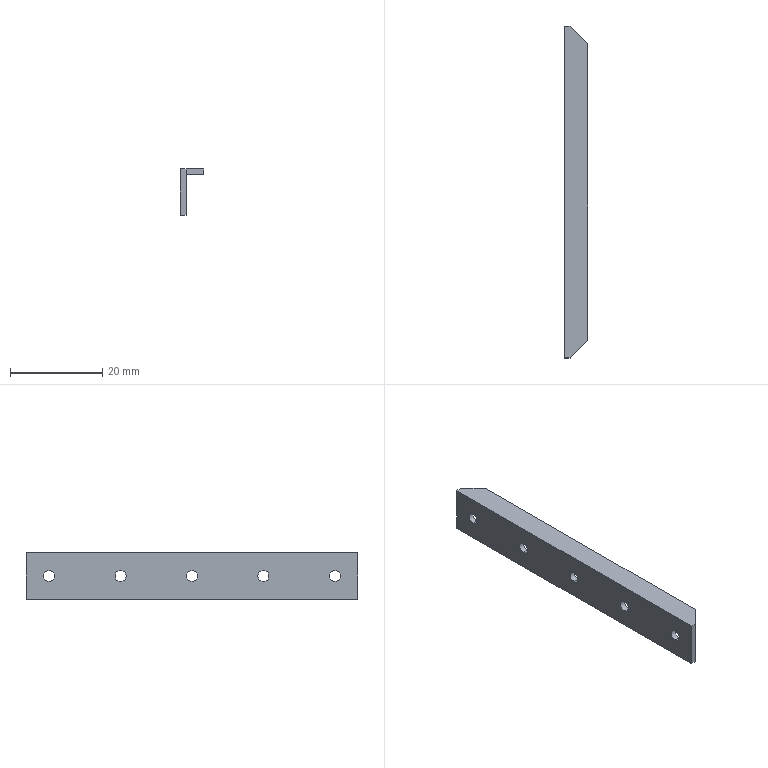Part | SolidWorks | features BaseBody 1 | 1 solid | 20 faces | box 5 x 72 x 10 mm | volume 1148 mm3 | cylinder 10 | plane 10 | commonest cylinder face diameters 2.4 x10
STEP:
#1=CARTESIAN_POINT('',(0.,20.5,-6.2));
#2=VERTEX_POINT('',#1);
#3=CARTESIAN_POINT('',(0.,20.5,-3.8));
#4=VERTEX_POINT('',#3);
#5=CARTESIAN_POINT('',(0.,20.5,-5.));
#6=DIRECTION('',(-1.,0.,0.));
#7=DIRECTION('',(0.,0.,-1.));
#8=AXIS2_PLACEMENT_3D('',#5,#6,#7);
#9=CIRCLE('',#8,1.2);
#10=EDGE_CURVE('',#2,#4,#9,.T.);
#11=ORIENTED_EDGE('',*,*,#10,.T.);
#12=CARTESIAN_POINT('',(1.2,20.5,-3.8));
#13=VERTEX_POINT('',#12);
#14=CARTESIAN_POINT('',(0.,20.5,-3.8));
#15=DIRECTION('',(1.,0.,0.));
#16=VECTOR('',#15,1000.);
#17=LINE('',#14,#16);
#18=EDGE_CURVE('',#4,#13,#17,.T.);
#19=ORIENTED_EDGE('',*,*,#18,.T.);
#20=CARTESIAN_POINT('',(1.2,20.5,-6.2));
#21=VERTEX_POINT('',#20);
#22=CARTESIAN_POINT('',(1.2,20.5,-5.));
#23=DIRECTION('',(1.,0.,0.));
#24=DIRECTION('',(0.,0.,-1.));
#25=AXIS2_PLACEMENT_3D('',#22,#23,#24);
#26=CIRCLE('',#25,1.2);
#27=EDGE_CURVE('',#13,#21,#26,.T.);
#28=ORIENTED_EDGE('',*,*,#27,.T.);
#29=CARTESIAN_POINT('',(0.,20.5,-6.2));
#30=DIRECTION('',(1.,0.,0.));
#31=VECTOR('',#30,1000.);
#32=LINE('',#29,#31);
#33=EDGE_CURVE('',#2,#21,#32,.T.);
#34=ORIENTED_EDGE('',*,*,#33,.F.);
#35=EDGE_LOOP('',(#11,#19,#28,#34));
#36=FACE_OUTER_BOUND('',#35,.T.);
#37=CARTESIAN_POINT('',(0.,20.5,-5.));
#38=DIRECTION('',(1.,0.,0.));
#39=DIRECTION('',(0.,0.,-1.));
#40=AXIS2_PLACEMENT_3D('',#37,#38,#39);
#41=CYLINDRICAL_SURFACE('',#40,1.2);
#42=ADVANCED_FACE('',(#36),#41,.F.);
#43=CARTESIAN_POINT('',(0.,67.,-6.2));
#44=VERTEX_POINT('',#43);
#45=CARTESIAN_POINT('',(0.,67.,-3.8));
#46=VERTEX_POINT('',#45);
#47=CARTESIAN_POINT('',(0.,67.,-5.));
#48=DIRECTION('',(-1.,0.,0.));
#49=DIRECTION('',(0.,0.,-1.));
#50=AXIS2_PLACEMENT_3D('',#47,#48,#49);
#51=CIRCLE('',#50,1.2);
#52=EDGE_CURVE('',#44,#46,#51,.T.);
#53=ORIENTED_EDGE('',*,*,#52,.T.);
#54=CARTESIAN_POINT('',(1.2,67.,-3.8));
#55=VERTEX_POINT('',#54);
#56=CARTESIAN_POINT('',(0.,67.,-3.8));
#57=DIRECTION('',(1.,0.,0.));
#58=VECTOR('',#57,1000.);
#59=LINE('',#56,#58);
#60=EDGE_CURVE('',#46,#55,#59,.T.);
#61=ORIENTED_EDGE('',*,*,#60,.T.);
#62=CARTESIAN_POINT('',(1.2,67.,-6.2));
#63=VERTEX_POINT('',#62);
#64=CARTESIAN_POINT('',(1.2,67.,-5.));
#65=DIRECTION('',(1.,0.,0.));
#66=DIRECTION('',(0.,0.,-1.));
#67=AXIS2_PLACEMENT_3D('',#64,#65,#66);
#68=CIRCLE('',#67,1.2);
#69=EDGE_CURVE('',#55,#63,#68,.T.);
#70=ORIENTED_EDGE('',*,*,#69,.T.);
#71=CARTESIAN_POINT('',(0.,67.,-6.2));
#72=DIRECTION('',(1.,0.,0.));
#73=VECTOR('',#72,1000.);
#74=LINE('',#71,#73);
#75=EDGE_CURVE('',#44,#63,#74,.T.);
#76=ORIENTED_EDGE('',*,*,#75,.F.);
#77=EDGE_LOOP('',(#53,#61,#70,#76));
#78=FACE_OUTER_BOUND('',#77,.T.);
#79=CARTESIAN_POINT('',(0.,67.,-5.));
#80=DIRECTION('',(1.,0.,0.));
#81=DIRECTION('',(0.,0.,-1.));
#82=AXIS2_PLACEMENT_3D('',#79,#80,#81);
#83=CYLINDRICAL_SURFACE('',#82,1.2);
#84=ADVANCED_FACE('',(#78),#83,.F.);
#85=CARTESIAN_POINT('',(0.,5.,-6.2));
#86=VERTEX_POINT('',#85);
#87=CARTESIAN_POINT('',(0.,5.,-3.8));
#88=VERTEX_POINT('',#87);
#89=CARTESIAN_POINT('',(0.,5.,-5.));
#90=DIRECTION('',(-1.,0.,0.));
#91=DIRECTION('',(0.,0.,-1.));
#92=AXIS2_PLACEMENT_3D('',#89,#90,#91);
#93=CIRCLE('',#92,1.2);
#94=EDGE_CURVE('',#86,#88,#93,.T.);
#95=ORIENTED_EDGE('',*,*,#94,.T.);
#96=CARTESIAN_POINT('',(1.2,5.,-3.8));
#97=VERTEX_POINT('',#96);
#98=CARTESIAN_POINT('',(0.,5.,-3.8));
#99=DIRECTION('',(1.,0.,0.));
#100=VECTOR('',#99,1000.);
#101=LINE('',#98,#100);
#102=EDGE_CURVE('',#88,#97,#101,.T.);
#103=ORIENTED_EDGE('',*,*,#102,.T.);
#104=CARTESIAN_POINT('',(1.2,5.,-6.2));
#105=VERTEX_POINT('',#104);
#106=CARTESIAN_POINT('',(1.2,5.,-5.));
#107=DIRECTION('',(1.,0.,0.));
#108=DIRECTION('',(0.,0.,-1.));
#109=AXIS2_PLACEMENT_3D('',#106,#107,#108);
#110=CIRCLE('',#109,1.2);
#111=EDGE_CURVE('',#97,#105,#110,.T.);
#112=ORIENTED_EDGE('',*,*,#111,.T.);
#113=CARTESIAN_POINT('',(0.,5.,-6.2));
#114=DIRECTION('',(1.,0.,0.));
#115=VECTOR('',#114,1000.);
#116=LINE('',#113,#115);
#117=EDGE_CURVE('',#86,#105,#116,.T.);
#118=ORIENTED_EDGE('',*,*,#117,.F.);
#119=EDGE_LOOP('',(#95,#103,#112,#118));
#120=FACE_OUTER_BOUND('',#119,.T.);
#121=CARTESIAN_POINT('',(0.,5.,-5.));
#122=DIRECTION('',(1.,0.,0.));
#123=DIRECTION('',(0.,0.,-1.));
#124=AXIS2_PLACEMENT_3D('',#121,#122,#123);
#125=CYLINDRICAL_SURFACE('',#124,1.2);
#126=ADVANCED_FACE('',(#120),#125,.F.);
#127=CARTESIAN_POINT('',(0.,36.,-6.2));
#128=VERTEX_POINT('',#127);
#129=CARTESIAN_POINT('',(0.,36.,-3.8));
#130=VERTEX_POINT('',#129);
#131=CARTESIAN_POINT('',(0.,36.,-5.));
#132=DIRECTION('',(-1.,0.,0.));
#133=DIRECTION('',(0.,0.,-1.));
#134=AXIS2_PLACEMENT_3D('',#131,#132,#133);
#135=CIRCLE('',#134,1.2);
#136=EDGE_CURVE('',#128,#130,#135,.T.);
#137=ORIENTED_EDGE('',*,*,#136,.T.);
#138=CARTESIAN_POINT('',(1.2,36.,-3.8));
#139=VERTEX_POINT('',#138);
#140=CARTESIAN_POINT('',(0.,36.,-3.8));
#141=DIRECTION('',(1.,0.,0.));
#142=VECTOR('',#141,1000.);
#143=LINE('',#140,#142);
#144=EDGE_CURVE('',#130,#139,#143,.T.);
#145=ORIENTED_EDGE('',*,*,#144,.T.);
#146=CARTESIAN_POINT('',(1.2,36.,-6.2));
#147=VERTEX_POINT('',#146);
#148=CARTESIAN_POINT('',(1.2,36.,-5.));
#149=DIRECTION('',(1.,0.,0.));
#150=DIRECTION('',(0.,0.,-1.));
#151=AXIS2_PLACEMENT_3D('',#148,#149,#150);
#152=CIRCLE('',#151,1.2);
#153=EDGE_CURVE('',#139,#147,#152,.T.);
#154=ORIENTED_EDGE('',*,*,#153,.T.);
#155=CARTESIAN_POINT('',(0.,36.,-6.2));
#156=DIRECTION('',(1.,0.,0.));
#157=VECTOR('',#156,1000.);
#158=LINE('',#155,#157);
#159=EDGE_CURVE('',#128,#147,#158,.T.);
#160=ORIENTED_EDGE('',*,*,#159,.F.);
#161=EDGE_LOOP('',(#137,#145,#154,#160));
#162=FACE_OUTER_BOUND('',#161,.T.);
#163=CARTESIAN_POINT('',(0.,36.,-5.));
#164=DIRECTION('',(1.,0.,0.));
#165=DIRECTION('',(0.,0.,-1.));
#166=AXIS2_PLACEMENT_3D('',#163,#164,#165);
#167=CYLINDRICAL_SURFACE('',#166,1.2);
#168=ADVANCED_FACE('',(#162),#167,.F.);
#169=CARTESIAN_POINT('',(0.,51.5,-6.2));
#170=VERTEX_POINT('',#169);
#171=CARTESIAN_POINT('',(0.,51.5,-3.8));
#172=VERTEX_POINT('',#171);
#173=CARTESIAN_POINT('',(0.,51.5,-5.));
#174=DIRECTION('',(-1.,0.,0.));
#175=DIRECTION('',(0.,0.,-1.));
#176=AXIS2_PLACEMENT_3D('',#173,#174,#175);
#177=CIRCLE('',#176,1.2);
#178=EDGE_CURVE('',#170,#172,#177,.T.);
#179=ORIENTED_EDGE('',*,*,#178,.T.);
#180=CARTESIAN_POINT('',(1.2,51.5,-3.8));
#181=VERTEX_POINT('',#180);
#182=CARTESIAN_POINT('',(0.,51.5,-3.8));
#183=DIRECTION('',(1.,0.,0.));
#184=VECTOR('',#183,1000.);
#185=LINE('',#182,#184);
#186=EDGE_CURVE('',#172,#181,#185,.T.);
#187=ORIENTED_EDGE('',*,*,#186,.T.);
#188=CARTESIAN_POINT('',(1.2,51.5,-6.2));
#189=VERTEX_POINT('',#188);
#190=CARTESIAN_POINT('',(1.2,51.5,-5.));
#191=DIRECTION('',(1.,0.,0.));
#192=DIRECTION('',(0.,0.,-1.));
#193=AXIS2_PLACEMENT_3D('',#190,#191,#192);
#194=CIRCLE('',#193,1.2);
#195=EDGE_CURVE('',#181,#189,#194,.T.);
#196=ORIENTED_EDGE('',*,*,#195,.T.);
#197=CARTESIAN_POINT('',(0.,51.5,-6.2));
#198=DIRECTION('',(1.,0.,0.));
#199=VECTOR('',#198,1000.);
#200=LINE('',#197,#199);
#201=EDGE_CURVE('',#170,#189,#200,.T.);
#202=ORIENTED_EDGE('',*,*,#201,.F.);
#203=EDGE_LOOP('',(#179,#187,#196,#202));
#204=FACE_OUTER_BOUND('',#203,.T.);
#205=CARTESIAN_POINT('',(0.,51.5,-5.));
#206=DIRECTION('',(1.,0.,0.));
#207=DIRECTION('',(0.,0.,-1.));
#208=AXIS2_PLACEMENT_3D('',#205,#206,#207);
#209=CYLINDRICAL_SURFACE('',#208,1.2);
#210=ADVANCED_FACE('',(#204),#209,.F.);
#211=ORIENTED_EDGE('',*,*,#18,.F.);
#212=CARTESIAN_POINT('',(0.,20.5,-5.));
#213=DIRECTION('',(-1.,0.,0.));
#214=DIRECTION('',(0.,0.,-1.));
#215=AXIS2_PLACEMENT_3D('',#212,#213,#214);
#216=CIRCLE('',#215,1.2);
#217=EDGE_CURVE('',#4,#2,#216,.T.);
#218=ORIENTED_EDGE('',*,*,#217,.T.);
#219=ORIENTED_EDGE('',*,*,#33,.T.);
#220=CARTESIAN_POINT('',(1.2,20.5,-5.));
#221=DIRECTION('',(1.,0.,0.));
#222=DIRECTION('',(0.,0.,-1.));
#223=AXIS2_PLACEMENT_3D('',#220,#221,#222);
#224=CIRCLE('',#223,1.2);
#225=EDGE_CURVE('',#21,#13,#224,.T.);
#226=ORIENTED_EDGE('',*,*,#225,.T.);
#227=EDGE_LOOP('',(#211,#218,#219,#226));
#228=FACE_OUTER_BOUND('',#227,.T.);
#229=CARTESIAN_POINT('',(0.,20.5,-5.));
#230=DIRECTION('',(1.,0.,0.));
#231=DIRECTION('',(0.,0.,-1.));
#232=AXIS2_PLACEMENT_3D('',#229,#230,#231);
#233=CYLINDRICAL_SURFACE('',#232,1.2);
#234=ADVANCED_FACE('',(#228),#233,.F.);
#235=CARTESIAN_POINT('',(1.2,67.,-5.));
#236=DIRECTION('',(1.,0.,0.));
#237=DIRECTION('',(0.,0.,-1.));
#238=AXIS2_PLACEMENT_3D('',#235,#236,#237);
#239=CIRCLE('',#238,1.2);
#240=EDGE_CURVE('',#63,#55,#239,.T.);
#241=ORIENTED_EDGE('',*,*,#240,.F.);
#242=ORIENTED_EDGE('',*,*,#69,.F.);
#243=EDGE_LOOP('',(#241,#242));
#244=FACE_BOUND('',#243,.T.);
#245=CARTESIAN_POINT('',(1.2,5.,-5.));
#246=DIRECTION('',(1.,0.,0.));
#247=DIRECTION('',(0.,0.,-1.));
#248=AXIS2_PLACEMENT_3D('',#245,#246,#247);
#249=CIRCLE('',#248,1.2);
#250=EDGE_CURVE('',#105,#97,#249,.T.);
#251=ORIENTED_EDGE('',*,*,#250,.F.);
#252=ORIENTED_EDGE('',*,*,#111,.F.);
#253=EDGE_LOOP('',(#251,#252));
#254=FACE_BOUND('',#253,.T.);
#255=CARTESIAN_POINT('',(1.2,36.,-5.));
#256=DIRECTION('',(1.,0.,0.));
#257=DIRECTION('',(0.,0.,-1.));
#258=AXIS2_PLACEMENT_3D('',#255,#256,#257);
#259=CIRCLE('',#258,1.2);
#260=EDGE_CURVE('',#147,#139,#259,.T.);
#261=ORIENTED_EDGE('',*,*,#260,.F.);
#262=ORIENTED_EDGE('',*,*,#153,.F.);
#263=EDGE_LOOP('',(#261,#262));
#264=FACE_BOUND('',#263,.T.);
#265=CARTESIAN_POINT('',(1.2,51.5,-5.));
#266=DIRECTION('',(1.,0.,0.));
#267=DIRECTION('',(0.,0.,-1.));
#268=AXIS2_PLACEMENT_3D('',#265,#266,#267);
#269=CIRCLE('',#268,1.2);
#270=EDGE_CURVE('',#189,#181,#269,.T.);
#271=ORIENTED_EDGE('',*,*,#270,.F.);
#272=ORIENTED_EDGE('',*,*,#195,.F.);
#273=EDGE_LOOP('',(#271,#272));
#274=FACE_BOUND('',#273,.T.);
#275=ORIENTED_EDGE('',*,*,#225,.F.);
#276=ORIENTED_EDGE('',*,*,#27,.F.);
#277=EDGE_LOOP('',(#275,#276));
#278=FACE_BOUND('',#277,.T.);
#279=CARTESIAN_POINT('',(1.2,72.,-10.));
#280=VERTEX_POINT('',#279);
#281=CARTESIAN_POINT('',(1.2,0.,-10.));
#282=VERTEX_POINT('',#281);
#283=CARTESIAN_POINT('',(1.2,36.,-10.));
#284=DIRECTION('',(0.,-1.,0.));
#285=VECTOR('',#284,1000.);
#286=LINE('',#283,#285);
#287=EDGE_CURVE('',#280,#282,#286,.T.);
#288=ORIENTED_EDGE('',*,*,#287,.F.);
#289=CARTESIAN_POINT('',(1.2,72.,-1.2));
#290=VERTEX_POINT('',#289);
#291=CARTESIAN_POINT('',(1.2,72.,-5.6));
#292=DIRECTION('',(0.,0.,-1.));
#293=VECTOR('',#292,1000.);
#294=LINE('',#291,#293);
#295=EDGE_CURVE('',#290,#280,#294,.T.);
#296=ORIENTED_EDGE('',*,*,#295,.F.);
#297=CARTESIAN_POINT('',(1.2,0.,-1.2));
#298=VERTEX_POINT('',#297);
#299=CARTESIAN_POINT('',(1.2,36.,-1.2));
#300=DIRECTION('',(0.,1.,0.));
#301=VECTOR('',#300,1000.);
#302=LINE('',#299,#301);
#303=EDGE_CURVE('',#298,#290,#302,.T.);
#304=ORIENTED_EDGE('',*,*,#303,.F.);
#305=CARTESIAN_POINT('',(1.2,0.,-5.6));
#306=DIRECTION('',(0.,0.,1.));
#307=VECTOR('',#306,1000.);
#308=LINE('',#305,#307);
#309=EDGE_CURVE('',#282,#298,#308,.T.);
#310=ORIENTED_EDGE('',*,*,#309,.F.);
#311=EDGE_LOOP('',(#288,#296,#304,#310));
#312=FACE_OUTER_BOUND('',#311,.T.);
#313=CARTESIAN_POINT('',(1.2,0.,-10.));
#314=DIRECTION('',(-1.,0.,0.));
#315=DIRECTION('',(0.,0.,1.));
#316=AXIS2_PLACEMENT_3D('',#313,#314,#315);
#317=PLANE('',#316);
#318=ADVANCED_FACE('',(#244,#254,#264,#274,#278,#312),#317,.F.);
#319=ORIENTED_EDGE('',*,*,#52,.F.);
#320=CARTESIAN_POINT('',(0.,67.,-5.));
#321=DIRECTION('',(-1.,0.,0.));
#322=DIRECTION('',(0.,0.,-1.));
#323=AXIS2_PLACEMENT_3D('',#320,#321,#322);
#324=CIRCLE('',#323,1.2);
#325=EDGE_CURVE('',#46,#44,#324,.T.);
#326=ORIENTED_EDGE('',*,*,#325,.F.);
#327=EDGE_LOOP('',(#319,#326));
#328=FACE_BOUND('',#327,.T.);
#329=ORIENTED_EDGE('',*,*,#94,.F.);
#330=CARTESIAN_POINT('',(0.,5.,-5.));
#331=DIRECTION('',(-1.,0.,0.));
#332=DIRECTION('',(0.,0.,-1.));
#333=AXIS2_PLACEMENT_3D('',#330,#331,#332);
#334=CIRCLE('',#333,1.2);
#335=EDGE_CURVE('',#88,#86,#334,.T.);
#336=ORIENTED_EDGE('',*,*,#335,.F.);
#337=EDGE_LOOP('',(#329,#336));
#338=FACE_BOUND('',#337,.T.);
#339=ORIENTED_EDGE('',*,*,#136,.F.);
#340=CARTESIAN_POINT('',(0.,36.,-5.));
#341=DIRECTION('',(-1.,0.,0.));
#342=DIRECTION('',(0.,0.,-1.));
#343=AXIS2_PLACEMENT_3D('',#340,#341,#342);
#344=CIRCLE('',#343,1.2);
#345=EDGE_CURVE('',#130,#128,#344,.T.);
#346=ORIENTED_EDGE('',*,*,#345,.F.);
#347=EDGE_LOOP('',(#339,#346));
#348=FACE_BOUND('',#347,.T.);
#349=ORIENTED_EDGE('',*,*,#178,.F.);
#350=CARTESIAN_POINT('',(0.,51.5,-5.));
#351=DIRECTION('',(-1.,0.,0.));
#352=DIRECTION('',(0.,0.,-1.));
#353=AXIS2_PLACEMENT_3D('',#350,#351,#352);
#354=CIRCLE('',#353,1.2);
#355=EDGE_CURVE('',#172,#170,#354,.T.);
#356=ORIENTED_EDGE('',*,*,#355,.F.);
#357=EDGE_LOOP('',(#349,#356));
#358=FACE_BOUND('',#357,.T.);
#359=ORIENTED_EDGE('',*,*,#10,.F.);
#360=ORIENTED_EDGE('',*,*,#217,.F.);
#361=EDGE_LOOP('',(#359,#360));
#362=FACE_BOUND('',#361,.T.);
#363=CARTESIAN_POINT('',(0.,72.,0.));
#364=VERTEX_POINT('',#363);
#365=CARTESIAN_POINT('',(0.,0.,0.));
#366=VERTEX_POINT('',#365);
#367=CARTESIAN_POINT('',(0.,36.,0.));
#368=DIRECTION('',(0.,-1.,0.));
#369=VECTOR('',#368,1000.);
#370=LINE('',#367,#369);
#371=EDGE_CURVE('',#364,#366,#370,.T.);
#372=ORIENTED_EDGE('',*,*,#371,.F.);
#373=CARTESIAN_POINT('',(0.,72.,-10.));
#374=VERTEX_POINT('',#373);
#375=CARTESIAN_POINT('',(0.,72.,-5.));
#376=DIRECTION('',(0.,0.,1.));
#377=VECTOR('',#376,1000.);
#378=LINE('',#375,#377);
#379=EDGE_CURVE('',#374,#364,#378,.T.);
#380=ORIENTED_EDGE('',*,*,#379,.F.);
#381=CARTESIAN_POINT('',(0.,0.,-10.));
#382=VERTEX_POINT('',#381);
#383=CARTESIAN_POINT('',(0.,36.,-10.));
#384=DIRECTION('',(0.,1.,0.));
#385=VECTOR('',#384,1000.);
#386=LINE('',#383,#385);
#387=EDGE_CURVE('',#382,#374,#386,.T.);
#388=ORIENTED_EDGE('',*,*,#387,.F.);
#389=CARTESIAN_POINT('',(0.,0.,-5.));
#390=DIRECTION('',(0.,0.,-1.));
#391=VECTOR('',#390,1000.);
#392=LINE('',#389,#391);
#393=EDGE_CURVE('',#366,#382,#392,.T.);
#394=ORIENTED_EDGE('',*,*,#393,.F.);
#395=EDGE_LOOP('',(#372,#380,#388,#394));
#396=FACE_OUTER_BOUND('',#395,.T.);
#397=CARTESIAN_POINT('',(0.,0.,0.));
#398=DIRECTION('',(1.,0.,0.));
#399=DIRECTION('',(0.,0.,-1.));
#400=AXIS2_PLACEMENT_3D('',#397,#398,#399);
#401=PLANE('',#400);
#402=ADVANCED_FACE('',(#328,#338,#348,#358,#362,#396),#401,.F.);
#403=ORIENTED_EDGE('',*,*,#60,.F.);
#404=ORIENTED_EDGE('',*,*,#325,.T.);
#405=ORIENTED_EDGE('',*,*,#75,.T.);
#406=ORIENTED_EDGE('',*,*,#240,.T.);
#407=EDGE_LOOP('',(#403,#404,#405,#406));
#408=FACE_OUTER_BOUND('',#407,.T.);
#409=CARTESIAN_POINT('',(0.,67.,-5.));
#410=DIRECTION('',(1.,0.,0.));
#411=DIRECTION('',(0.,0.,-1.));
#412=AXIS2_PLACEMENT_3D('',#409,#410,#411);
#413=CYLINDRICAL_SURFACE('',#412,1.2);
#414=ADVANCED_FACE('',(#408),#413,.F.);
#415=ORIENTED_EDGE('',*,*,#102,.F.);
#416=ORIENTED_EDGE('',*,*,#335,.T.);
#417=ORIENTED_EDGE('',*,*,#117,.T.);
#418=ORIENTED_EDGE('',*,*,#250,.T.);
#419=EDGE_LOOP('',(#415,#416,#417,#418));
#420=FACE_OUTER_BOUND('',#419,.T.);
#421=CARTESIAN_POINT('',(0.,5.,-5.));
#422=DIRECTION('',(1.,0.,0.));
#423=DIRECTION('',(0.,0.,-1.));
#424=AXIS2_PLACEMENT_3D('',#421,#422,#423);
#425=CYLINDRICAL_SURFACE('',#424,1.2);
#426=ADVANCED_FACE('',(#420),#425,.F.);
#427=ORIENTED_EDGE('',*,*,#144,.F.);
#428=ORIENTED_EDGE('',*,*,#345,.T.);
#429=ORIENTED_EDGE('',*,*,#159,.T.);
#430=ORIENTED_EDGE('',*,*,#260,.T.);
#431=EDGE_LOOP('',(#427,#428,#429,#430));
#432=FACE_OUTER_BOUND('',#431,.T.);
#433=CARTESIAN_POINT('',(0.,36.,-5.));
#434=DIRECTION('',(1.,0.,0.));
#435=DIRECTION('',(0.,0.,-1.));
#436=AXIS2_PLACEMENT_3D('',#433,#434,#435);
#437=CYLINDRICAL_SURFACE('',#436,1.2);
#438=ADVANCED_FACE('',(#432),#437,.F.);
#439=ORIENTED_EDGE('',*,*,#186,.F.);
#440=ORIENTED_EDGE('',*,*,#355,.T.);
#441=ORIENTED_EDGE('',*,*,#201,.T.);
#442=ORIENTED_EDGE('',*,*,#270,.T.);
#443=EDGE_LOOP('',(#439,#440,#441,#442));
#444=FACE_OUTER_BOUND('',#443,.T.);
#445=CARTESIAN_POINT('',(0.,51.5,-5.));
#446=DIRECTION('',(1.,0.,0.));
#447=DIRECTION('',(0.,0.,-1.));
#448=AXIS2_PLACEMENT_3D('',#445,#446,#447);
#449=CYLINDRICAL_SURFACE('',#448,1.2);
#450=ADVANCED_FACE('',(#444),#449,.F.);
#451=CARTESIAN_POINT('',(0.6,0.,-10.));
#452=DIRECTION('',(1.,0.,0.));
#453=VECTOR('',#452,1000.);
#454=LINE('',#451,#453);
#455=EDGE_CURVE('',#382,#282,#454,.T.);
#456=ORIENTED_EDGE('',*,*,#455,.T.);
#457=ORIENTED_EDGE('',*,*,#309,.T.);
#458=CARTESIAN_POINT('',(1.2,0.,0.));
#459=VERTEX_POINT('',#458);
#460=CARTESIAN_POINT('',(1.2,0.,-0.6));
#461=DIRECTION('',(0.,0.,1.));
#462=VECTOR('',#461,1000.);
#463=LINE('',#460,#462);
#464=EDGE_CURVE('',#298,#459,#463,.T.);
#465=ORIENTED_EDGE('',*,*,#464,.T.);
#466=CARTESIAN_POINT('',(0.6,0.,0.));
#467=DIRECTION('',(-1.,0.,0.));
#468=VECTOR('',#467,1000.);
#469=LINE('',#466,#468);
#470=EDGE_CURVE('',#459,#366,#469,.T.);
#471=ORIENTED_EDGE('',*,*,#470,.T.);
#472=ORIENTED_EDGE('',*,*,#393,.T.);
#473=EDGE_LOOP('',(#456,#457,#465,#471,#472));
#474=FACE_OUTER_BOUND('',#473,.T.);
#475=CARTESIAN_POINT('',(0.,0.,0.));
#476=DIRECTION('',(0.,-1.,0.));
#477=DIRECTION('',(0.,0.,-1.));
#478=AXIS2_PLACEMENT_3D('',#475,#476,#477);
#479=PLANE('',#478);
#480=ADVANCED_FACE('',(#474),#479,.T.);
#481=ORIENTED_EDGE('',*,*,#387,.T.);
#482=CARTESIAN_POINT('',(0.6,72.,-10.));
#483=DIRECTION('',(-1.,0.,0.));
#484=VECTOR('',#483,1000.);
#485=LINE('',#482,#484);
#486=EDGE_CURVE('',#280,#374,#485,.T.);
#487=ORIENTED_EDGE('',*,*,#486,.F.);
#488=ORIENTED_EDGE('',*,*,#287,.T.);
#489=ORIENTED_EDGE('',*,*,#455,.F.);
#490=EDGE_LOOP('',(#481,#487,#488,#489));
#491=FACE_OUTER_BOUND('',#490,.T.);
#492=CARTESIAN_POINT('',(0.,0.,-10.));
#493=DIRECTION('',(0.,0.,1.));
#494=DIRECTION('',(1.,0.,0.));
#495=AXIS2_PLACEMENT_3D('',#492,#493,#494);
#496=PLANE('',#495);
#497=ADVANCED_FACE('',(#491),#496,.F.);
#498=CARTESIAN_POINT('',(1.2,72.,0.));
#499=VERTEX_POINT('',#498);
#500=CARTESIAN_POINT('',(1.2,72.,-0.6));
#501=DIRECTION('',(0.,0.,-1.));
#502=VECTOR('',#501,1000.);
#503=LINE('',#500,#502);
#504=EDGE_CURVE('',#499,#290,#503,.T.);
#505=ORIENTED_EDGE('',*,*,#504,.T.);
#506=ORIENTED_EDGE('',*,*,#295,.T.);
#507=ORIENTED_EDGE('',*,*,#486,.T.);
#508=ORIENTED_EDGE('',*,*,#379,.T.);
#509=CARTESIAN_POINT('',(0.6,72.,0.));
#510=DIRECTION('',(-1.,0.,0.));
#511=VECTOR('',#510,1000.);
#512=LINE('',#509,#511);
#513=EDGE_CURVE('',#499,#364,#512,.T.);
#514=ORIENTED_EDGE('',*,*,#513,.F.);
#515=EDGE_LOOP('',(#505,#506,#507,#508,#514));
#516=FACE_OUTER_BOUND('',#515,.T.);
#517=CARTESIAN_POINT('',(0.,72.,0.));
#518=DIRECTION('',(0.,-1.,0.));
#519=DIRECTION('',(0.,0.,-1.));
#520=AXIS2_PLACEMENT_3D('',#517,#518,#519);
#521=PLANE('',#520);
#522=ADVANCED_FACE('',(#516),#521,.F.);
#523=CARTESIAN_POINT('',(5.,3.8,-1.2));
#524=VERTEX_POINT('',#523);
#525=CARTESIAN_POINT('',(5.,3.8,-1.2));
#526=DIRECTION('',(0.7071,0.7071,0.));
#527=VECTOR('',#526,1000.);
#528=LINE('',#525,#527);
#529=EDGE_CURVE('',#298,#524,#528,.T.);
#530=ORIENTED_EDGE('',*,*,#529,.F.);
#531=ORIENTED_EDGE('',*,*,#303,.T.);
#532=CARTESIAN_POINT('',(5.,68.2,-1.2));
#533=VERTEX_POINT('',#532);
#534=CARTESIAN_POINT('',(1.2,72.,-1.2));
#535=DIRECTION('',(-0.7071,0.7071,0.));
#536=VECTOR('',#535,1000.);
#537=LINE('',#534,#536);
#538=EDGE_CURVE('',#533,#290,#537,.T.);
#539=ORIENTED_EDGE('',*,*,#538,.F.);
#540=CARTESIAN_POINT('',(5.,36.,-1.2));
#541=DIRECTION('',(0.,1.,0.));
#542=VECTOR('',#541,1000.);
#543=LINE('',#540,#542);
#544=EDGE_CURVE('',#524,#533,#543,.T.);
#545=ORIENTED_EDGE('',*,*,#544,.F.);
#546=EDGE_LOOP('',(#530,#531,#539,#545));
#547=FACE_OUTER_BOUND('',#546,.T.);
#548=CARTESIAN_POINT('',(1.2,-0.432,-1.2));
#549=DIRECTION('',(0.,0.,1.));
#550=DIRECTION('',(1.,0.,0.));
#551=AXIS2_PLACEMENT_3D('',#548,#549,#550);
#552=PLANE('',#551);
#553=ADVANCED_FACE('',(#547),#552,.F.);
#554=CARTESIAN_POINT('',(5.,3.8,0.));
#555=VERTEX_POINT('',#554);
#556=CARTESIAN_POINT('',(5.,3.8,0.));
#557=DIRECTION('',(-0.7071,-0.7071,0.));
#558=VECTOR('',#557,1000.);
#559=LINE('',#556,#558);
#560=EDGE_CURVE('',#555,#459,#559,.T.);
#561=ORIENTED_EDGE('',*,*,#560,.F.);
#562=CARTESIAN_POINT('',(5.,68.2,0.));
#563=VERTEX_POINT('',#562);
#564=CARTESIAN_POINT('',(5.,36.,0.));
#565=DIRECTION('',(0.,-1.,0.));
#566=VECTOR('',#565,1000.);
#567=LINE('',#564,#566);
#568=EDGE_CURVE('',#563,#555,#567,.T.);
#569=ORIENTED_EDGE('',*,*,#568,.F.);
#570=CARTESIAN_POINT('',(1.2,72.,0.));
#571=DIRECTION('',(0.7071,-0.7071,0.));
#572=VECTOR('',#571,1000.);
#573=LINE('',#570,#572);
#574=EDGE_CURVE('',#499,#563,#573,.T.);
#575=ORIENTED_EDGE('',*,*,#574,.F.);
#576=ORIENTED_EDGE('',*,*,#513,.T.);
#577=ORIENTED_EDGE('',*,*,#371,.T.);
#578=ORIENTED_EDGE('',*,*,#470,.F.);
#579=EDGE_LOOP('',(#561,#569,#575,#576,#577,#578));
#580=FACE_OUTER_BOUND('',#579,.T.);
#581=CARTESIAN_POINT('',(5.,0.,0.));
#582=DIRECTION('',(0.,0.,-1.));
#583=DIRECTION('',(-1.,0.,0.));
#584=AXIS2_PLACEMENT_3D('',#581,#582,#583);
#585=PLANE('',#584);
#586=ADVANCED_FACE('',(#580),#585,.F.);
#587=CARTESIAN_POINT('',(5.,3.8,-0.6));
#588=DIRECTION('',(0.,0.,1.));
#589=VECTOR('',#588,1000.);
#590=LINE('',#587,#589);
#591=EDGE_CURVE('',#524,#555,#590,.T.);
#592=ORIENTED_EDGE('',*,*,#591,.F.);
#593=ORIENTED_EDGE('',*,*,#544,.T.);
#594=CARTESIAN_POINT('',(5.,68.2,-0.6));
#595=DIRECTION('',(0.,0.,-1.));
#596=VECTOR('',#595,1000.);
#597=LINE('',#594,#596);
#598=EDGE_CURVE('',#563,#533,#597,.T.);
#599=ORIENTED_EDGE('',*,*,#598,.F.);
#600=ORIENTED_EDGE('',*,*,#568,.T.);
#601=EDGE_LOOP('',(#592,#593,#599,#600));
#602=FACE_OUTER_BOUND('',#601,.T.);
#603=CARTESIAN_POINT('',(5.,3.8,-1.2));
#604=DIRECTION('',(-1.,0.,0.));
#605=DIRECTION('',(0.,0.,1.));
#606=AXIS2_PLACEMENT_3D('',#603,#604,#605);
#607=PLANE('',#606);
#608=ADVANCED_FACE('',(#602),#607,.F.);
#609=ORIENTED_EDGE('',*,*,#529,.T.);
#610=ORIENTED_EDGE('',*,*,#591,.T.);
#611=ORIENTED_EDGE('',*,*,#560,.T.);
#612=ORIENTED_EDGE('',*,*,#464,.F.);
#613=EDGE_LOOP('',(#609,#610,#611,#612));
#614=FACE_OUTER_BOUND('',#613,.T.);
#615=CARTESIAN_POINT('',(5.,3.8,-1.2));
#616=DIRECTION('',(-0.7071,0.7071,0.));
#617=DIRECTION('',(-0.7071,-0.7071,0.));
#618=AXIS2_PLACEMENT_3D('',#615,#616,#617);
#619=PLANE('',#618);
#620=ADVANCED_FACE('',(#614),#619,.F.);
#621=ORIENTED_EDGE('',*,*,#538,.T.);
#622=ORIENTED_EDGE('',*,*,#504,.F.);
#623=ORIENTED_EDGE('',*,*,#574,.T.);
#624=ORIENTED_EDGE('',*,*,#598,.T.);
#625=EDGE_LOOP('',(#621,#622,#623,#624));
#626=FACE_OUTER_BOUND('',#625,.T.);
#627=CARTESIAN_POINT('',(1.2,72.,-1.2));
#628=DIRECTION('',(-0.7071,-0.7071,0.));
#629=DIRECTION('',(0.7071,-0.7071,0.));
#630=AXIS2_PLACEMENT_3D('',#627,#628,#629);
#631=PLANE('',#630);
#632=ADVANCED_FACE('',(#626),#631,.F.);
#633=CLOSED_SHELL('',(#42,#84,#126,#168,#210,#234,#318,#402,#414,#426,#438,#450,#480,#497,#522,#553,#586,#608,#620,#632));
#634=MANIFOLD_SOLID_BREP('',#633);
#635=CARTESIAN_POINT('',(0.,0.,0.));
#636=DIRECTION('',(0.,0.,1.));
#637=DIRECTION('',(1.,0.,0.));
#638=AXIS2_PLACEMENT_3D('',#635,#636,#637);
#639=(LENGTH_UNIT()NAMED_UNIT(*)SI_UNIT(.MILLI.,.METRE.));
#640=UNCERTAINTY_MEASURE_WITH_UNIT(LENGTH_MEASURE(0.00001),#639,'','');
#641=(NAMED_UNIT(*)PLANE_ANGLE_UNIT()SI_UNIT($,.RADIAN.));
#642=(NAMED_UNIT(*)SI_UNIT($,.STERADIAN.)SOLID_ANGLE_UNIT());
#643=(GEOMETRIC_REPRESENTATION_CONTEXT(3)GLOBAL_UNCERTAINTY_ASSIGNED_CONTEXT((#640))GLOBAL_UNIT_ASSIGNED_CONTEXT((#639,#641,#642))REPRESENTATION_CONTEXT('',''));
#644=ADVANCED_BREP_SHAPE_REPRESENTATION('',(#634,#638),#643);